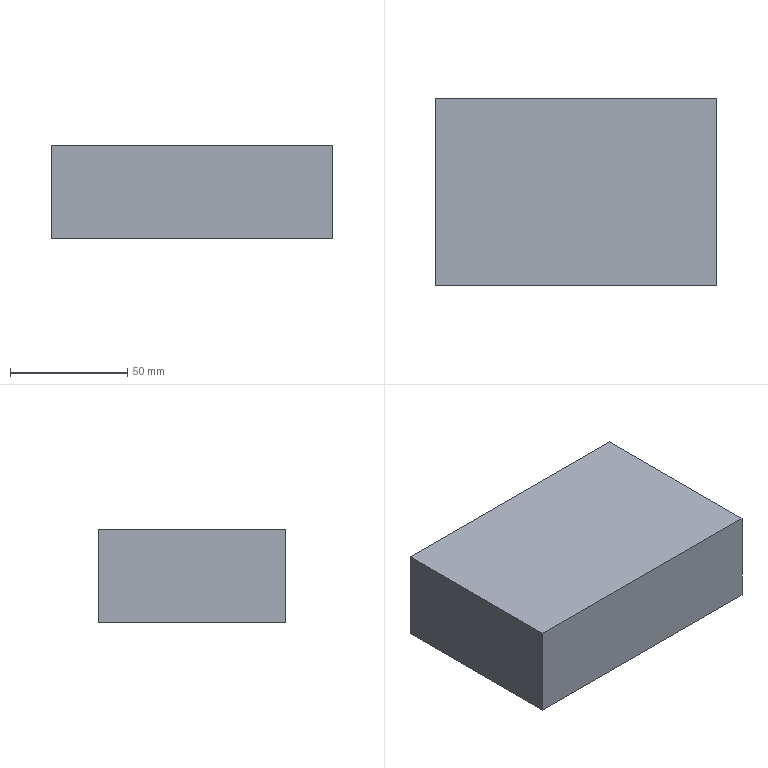Part | SolidWorks | features ICE 2, Extrusion 1 | 1 solid | 11 faces | box 120 x 80 x 40 mm | volume 204000 mm3 | plane 11
STEP:
#1=CARTESIAN_POINT('',(60.,40.,0.));
#2=VERTEX_POINT('',#1);
#3=CARTESIAN_POINT('',(60.,40.,40.));
#4=VERTEX_POINT('',#3);
#5=CARTESIAN_POINT('',(60.,40.,0.));
#6=DIRECTION('',(0.,0.,1.));
#7=VECTOR('',#6,1000.);
#8=LINE('',#5,#7);
#9=EDGE_CURVE('',#2,#4,#8,.T.);
#10=ORIENTED_EDGE('',*,*,#9,.T.);
#11=CARTESIAN_POINT('',(60.,-40.,40.));
#12=VERTEX_POINT('',#11);
#13=CARTESIAN_POINT('',(60.,-40.,40.));
#14=DIRECTION('',(0.,1.,0.));
#15=VECTOR('',#14,1000.);
#16=LINE('',#13,#15);
#17=EDGE_CURVE('',#12,#4,#16,.T.);
#18=ORIENTED_EDGE('',*,*,#17,.F.);
#19=CARTESIAN_POINT('',(60.,-40.,0.));
#20=VERTEX_POINT('',#19);
#21=CARTESIAN_POINT('',(60.,-40.,0.));
#22=DIRECTION('',(0.,0.,1.));
#23=VECTOR('',#22,1000.);
#24=LINE('',#21,#23);
#25=EDGE_CURVE('',#20,#12,#24,.T.);
#26=ORIENTED_EDGE('',*,*,#25,.F.);
#27=CARTESIAN_POINT('',(60.,-40.,0.));
#28=DIRECTION('',(0.,1.,0.));
#29=VECTOR('',#28,1000.);
#30=LINE('',#27,#29);
#31=EDGE_CURVE('',#20,#2,#30,.T.);
#32=ORIENTED_EDGE('',*,*,#31,.T.);
#33=EDGE_LOOP('',(#10,#18,#26,#32));
#34=FACE_OUTER_BOUND('',#33,.T.);
#35=CARTESIAN_POINT('',(60.,-40.,0.));
#36=DIRECTION('',(1.,0.,0.));
#37=DIRECTION('',(0.,0.,-1.));
#38=AXIS2_PLACEMENT_3D('',#35,#36,#37);
#39=PLANE('',#38);
#40=ADVANCED_FACE('',(#34),#39,.T.);
#41=ORIENTED_EDGE('',*,*,#25,.T.);
#42=CARTESIAN_POINT('',(-60.,-40.,40.));
#43=VERTEX_POINT('',#42);
#44=CARTESIAN_POINT('',(-60.,-40.,40.));
#45=DIRECTION('',(1.,0.,0.));
#46=VECTOR('',#45,1000.);
#47=LINE('',#44,#46);
#48=EDGE_CURVE('',#43,#12,#47,.T.);
#49=ORIENTED_EDGE('',*,*,#48,.F.);
#50=CARTESIAN_POINT('',(-60.,-40.,0.));
#51=VERTEX_POINT('',#50);
#52=CARTESIAN_POINT('',(-60.,-40.,0.));
#53=DIRECTION('',(0.,0.,1.));
#54=VECTOR('',#53,1000.);
#55=LINE('',#52,#54);
#56=EDGE_CURVE('',#51,#43,#55,.T.);
#57=ORIENTED_EDGE('',*,*,#56,.F.);
#58=CARTESIAN_POINT('',(-60.,-40.,0.));
#59=DIRECTION('',(1.,0.,0.));
#60=VECTOR('',#59,1000.);
#61=LINE('',#58,#60);
#62=EDGE_CURVE('',#51,#20,#61,.T.);
#63=ORIENTED_EDGE('',*,*,#62,.T.);
#64=EDGE_LOOP('',(#41,#49,#57,#63));
#65=FACE_OUTER_BOUND('',#64,.T.);
#66=CARTESIAN_POINT('',(-60.,-40.,0.));
#67=DIRECTION('',(0.,-1.,0.));
#68=DIRECTION('',(1.,0.,0.));
#69=AXIS2_PLACEMENT_3D('',#66,#67,#68);
#70=PLANE('',#69);
#71=ADVANCED_FACE('',(#65),#70,.T.);
#72=ORIENTED_EDGE('',*,*,#56,.T.);
#73=CARTESIAN_POINT('',(-60.,40.,40.));
#74=VERTEX_POINT('',#73);
#75=CARTESIAN_POINT('',(-60.,40.,40.));
#76=DIRECTION('',(0.,-1.,0.));
#77=VECTOR('',#76,1000.);
#78=LINE('',#75,#77);
#79=EDGE_CURVE('',#74,#43,#78,.T.);
#80=ORIENTED_EDGE('',*,*,#79,.F.);
#81=CARTESIAN_POINT('',(-60.,40.,0.));
#82=VERTEX_POINT('',#81);
#83=CARTESIAN_POINT('',(-60.,40.,0.));
#84=DIRECTION('',(0.,0.,1.));
#85=VECTOR('',#84,1000.);
#86=LINE('',#83,#85);
#87=EDGE_CURVE('',#82,#74,#86,.T.);
#88=ORIENTED_EDGE('',*,*,#87,.F.);
#89=CARTESIAN_POINT('',(-60.,40.,0.));
#90=DIRECTION('',(0.,-1.,0.));
#91=VECTOR('',#90,1000.);
#92=LINE('',#89,#91);
#93=EDGE_CURVE('',#82,#51,#92,.T.);
#94=ORIENTED_EDGE('',*,*,#93,.T.);
#95=EDGE_LOOP('',(#72,#80,#88,#94));
#96=FACE_OUTER_BOUND('',#95,.T.);
#97=CARTESIAN_POINT('',(-60.,40.,0.));
#98=DIRECTION('',(-1.,0.,0.));
#99=DIRECTION('',(0.,-1.,0.));
#100=AXIS2_PLACEMENT_3D('',#97,#98,#99);
#101=PLANE('',#100);
#102=ADVANCED_FACE('',(#96),#101,.T.);
#103=ORIENTED_EDGE('',*,*,#87,.T.);
#104=CARTESIAN_POINT('',(60.,40.,40.));
#105=DIRECTION('',(-1.,0.,0.));
#106=VECTOR('',#105,1000.);
#107=LINE('',#104,#106);
#108=EDGE_CURVE('',#4,#74,#107,.T.);
#109=ORIENTED_EDGE('',*,*,#108,.F.);
#110=ORIENTED_EDGE('',*,*,#9,.F.);
#111=CARTESIAN_POINT('',(60.,40.,0.));
#112=DIRECTION('',(-1.,0.,0.));
#113=VECTOR('',#112,1000.);
#114=LINE('',#111,#113);
#115=EDGE_CURVE('',#2,#82,#114,.T.);
#116=ORIENTED_EDGE('',*,*,#115,.T.);
#117=EDGE_LOOP('',(#103,#109,#110,#116));
#118=FACE_OUTER_BOUND('',#117,.T.);
#119=CARTESIAN_POINT('',(60.,40.,0.));
#120=DIRECTION('',(0.,1.,0.));
#121=DIRECTION('',(-1.,0.,0.));
#122=AXIS2_PLACEMENT_3D('',#119,#120,#121);
#123=PLANE('',#122);
#124=ADVANCED_FACE('',(#118),#123,.T.);
#125=CARTESIAN_POINT('',(50.,-30.,0.));
#126=VERTEX_POINT('',#125);
#127=CARTESIAN_POINT('',(50.,30.,0.));
#128=VERTEX_POINT('',#127);
#129=CARTESIAN_POINT('',(50.,-30.,0.));
#130=DIRECTION('',(0.,1.,0.));
#131=VECTOR('',#130,1000.);
#132=LINE('',#129,#131);
#133=EDGE_CURVE('',#126,#128,#132,.T.);
#134=ORIENTED_EDGE('',*,*,#133,.T.);
#135=CARTESIAN_POINT('',(-50.,30.,0.));
#136=VERTEX_POINT('',#135);
#137=CARTESIAN_POINT('',(50.,30.,0.));
#138=DIRECTION('',(-1.,0.,0.));
#139=VECTOR('',#138,1000.);
#140=LINE('',#137,#139);
#141=EDGE_CURVE('',#128,#136,#140,.T.);
#142=ORIENTED_EDGE('',*,*,#141,.T.);
#143=CARTESIAN_POINT('',(-50.,-30.,0.));
#144=VERTEX_POINT('',#143);
#145=CARTESIAN_POINT('',(-50.,30.,0.));
#146=DIRECTION('',(0.,-1.,0.));
#147=VECTOR('',#146,1000.);
#148=LINE('',#145,#147);
#149=EDGE_CURVE('',#136,#144,#148,.T.);
#150=ORIENTED_EDGE('',*,*,#149,.T.);
#151=CARTESIAN_POINT('',(-50.,-30.,0.));
#152=DIRECTION('',(1.,0.,0.));
#153=VECTOR('',#152,1000.);
#154=LINE('',#151,#153);
#155=EDGE_CURVE('',#144,#126,#154,.T.);
#156=ORIENTED_EDGE('',*,*,#155,.T.);
#157=EDGE_LOOP('',(#134,#142,#150,#156));
#158=FACE_BOUND('',#157,.T.);
#159=ORIENTED_EDGE('',*,*,#31,.F.);
#160=ORIENTED_EDGE('',*,*,#62,.F.);
#161=ORIENTED_EDGE('',*,*,#93,.F.);
#162=ORIENTED_EDGE('',*,*,#115,.F.);
#163=EDGE_LOOP('',(#159,#160,#161,#162));
#164=FACE_OUTER_BOUND('',#163,.T.);
#165=CARTESIAN_POINT('',(0.,0.,0.));
#166=DIRECTION('',(0.,0.,1.));
#167=DIRECTION('',(1.,0.,0.));
#168=AXIS2_PLACEMENT_3D('',#165,#166,#167);
#169=PLANE('',#168);
#170=ADVANCED_FACE('',(#158,#164),#169,.F.);
#171=CARTESIAN_POINT('',(50.,30.,30.));
#172=VERTEX_POINT('',#171);
#173=CARTESIAN_POINT('',(-50.,30.,30.));
#174=VERTEX_POINT('',#173);
#175=CARTESIAN_POINT('',(50.,30.,30.));
#176=DIRECTION('',(-1.,0.,0.));
#177=VECTOR('',#176,1000.);
#178=LINE('',#175,#177);
#179=EDGE_CURVE('',#172,#174,#178,.T.);
#180=ORIENTED_EDGE('',*,*,#179,.T.);
#181=CARTESIAN_POINT('',(-50.,30.,0.));
#182=DIRECTION('',(0.,0.,1.));
#183=VECTOR('',#182,1000.);
#184=LINE('',#181,#183);
#185=EDGE_CURVE('',#136,#174,#184,.T.);
#186=ORIENTED_EDGE('',*,*,#185,.F.);
#187=ORIENTED_EDGE('',*,*,#141,.F.);
#188=CARTESIAN_POINT('',(50.,30.,0.));
#189=DIRECTION('',(0.,0.,1.));
#190=VECTOR('',#189,1000.);
#191=LINE('',#188,#190);
#192=EDGE_CURVE('',#128,#172,#191,.T.);
#193=ORIENTED_EDGE('',*,*,#192,.T.);
#194=EDGE_LOOP('',(#180,#186,#187,#193));
#195=FACE_OUTER_BOUND('',#194,.T.);
#196=CARTESIAN_POINT('',(50.,30.,0.));
#197=DIRECTION('',(0.,1.,0.));
#198=DIRECTION('',(-1.,0.,0.));
#199=AXIS2_PLACEMENT_3D('',#196,#197,#198);
#200=PLANE('',#199);
#201=ADVANCED_FACE('',(#195),#200,.F.);
#202=CARTESIAN_POINT('',(50.,-30.,30.));
#203=VERTEX_POINT('',#202);
#204=CARTESIAN_POINT('',(50.,-30.,30.));
#205=DIRECTION('',(0.,1.,0.));
#206=VECTOR('',#205,1000.);
#207=LINE('',#204,#206);
#208=EDGE_CURVE('',#203,#172,#207,.T.);
#209=ORIENTED_EDGE('',*,*,#208,.T.);
#210=ORIENTED_EDGE('',*,*,#192,.F.);
#211=ORIENTED_EDGE('',*,*,#133,.F.);
#212=CARTESIAN_POINT('',(50.,-30.,0.));
#213=DIRECTION('',(0.,0.,1.));
#214=VECTOR('',#213,1000.);
#215=LINE('',#212,#214);
#216=EDGE_CURVE('',#126,#203,#215,.T.);
#217=ORIENTED_EDGE('',*,*,#216,.T.);
#218=EDGE_LOOP('',(#209,#210,#211,#217));
#219=FACE_OUTER_BOUND('',#218,.T.);
#220=CARTESIAN_POINT('',(50.,-30.,0.));
#221=DIRECTION('',(1.,0.,0.));
#222=DIRECTION('',(0.,0.,-1.));
#223=AXIS2_PLACEMENT_3D('',#220,#221,#222);
#224=PLANE('',#223);
#225=ADVANCED_FACE('',(#219),#224,.F.);
#226=CARTESIAN_POINT('',(-50.,-30.,30.));
#227=VERTEX_POINT('',#226);
#228=CARTESIAN_POINT('',(-50.,-30.,30.));
#229=DIRECTION('',(1.,0.,0.));
#230=VECTOR('',#229,1000.);
#231=LINE('',#228,#230);
#232=EDGE_CURVE('',#227,#203,#231,.T.);
#233=ORIENTED_EDGE('',*,*,#232,.T.);
#234=ORIENTED_EDGE('',*,*,#216,.F.);
#235=ORIENTED_EDGE('',*,*,#155,.F.);
#236=CARTESIAN_POINT('',(-50.,-30.,0.));
#237=DIRECTION('',(0.,0.,1.));
#238=VECTOR('',#237,1000.);
#239=LINE('',#236,#238);
#240=EDGE_CURVE('',#144,#227,#239,.T.);
#241=ORIENTED_EDGE('',*,*,#240,.T.);
#242=EDGE_LOOP('',(#233,#234,#235,#241));
#243=FACE_OUTER_BOUND('',#242,.T.);
#244=CARTESIAN_POINT('',(-50.,-30.,0.));
#245=DIRECTION('',(0.,-1.,0.));
#246=DIRECTION('',(1.,0.,0.));
#247=AXIS2_PLACEMENT_3D('',#244,#245,#246);
#248=PLANE('',#247);
#249=ADVANCED_FACE('',(#243),#248,.F.);
#250=CARTESIAN_POINT('',(-50.,30.,30.));
#251=DIRECTION('',(0.,-1.,0.));
#252=VECTOR('',#251,1000.);
#253=LINE('',#250,#252);
#254=EDGE_CURVE('',#174,#227,#253,.T.);
#255=ORIENTED_EDGE('',*,*,#254,.T.);
#256=ORIENTED_EDGE('',*,*,#240,.F.);
#257=ORIENTED_EDGE('',*,*,#149,.F.);
#258=ORIENTED_EDGE('',*,*,#185,.T.);
#259=EDGE_LOOP('',(#255,#256,#257,#258));
#260=FACE_OUTER_BOUND('',#259,.T.);
#261=CARTESIAN_POINT('',(-50.,30.,0.));
#262=DIRECTION('',(-1.,0.,0.));
#263=DIRECTION('',(0.,0.,1.));
#264=AXIS2_PLACEMENT_3D('',#261,#262,#263);
#265=PLANE('',#264);
#266=ADVANCED_FACE('',(#260),#265,.F.);
#267=ORIENTED_EDGE('',*,*,#179,.F.);
#268=ORIENTED_EDGE('',*,*,#208,.F.);
#269=ORIENTED_EDGE('',*,*,#232,.F.);
#270=ORIENTED_EDGE('',*,*,#254,.F.);
#271=EDGE_LOOP('',(#267,#268,#269,#270));
#272=FACE_OUTER_BOUND('',#271,.T.);
#273=CARTESIAN_POINT('',(0.,0.,30.));
#274=DIRECTION('',(0.,0.,1.));
#275=DIRECTION('',(1.,0.,0.));
#276=AXIS2_PLACEMENT_3D('',#273,#274,#275);
#277=PLANE('',#276);
#278=ADVANCED_FACE('',(#272),#277,.F.);
#279=ORIENTED_EDGE('',*,*,#48,.T.);
#280=ORIENTED_EDGE('',*,*,#17,.T.);
#281=ORIENTED_EDGE('',*,*,#108,.T.);
#282=ORIENTED_EDGE('',*,*,#79,.T.);
#283=EDGE_LOOP('',(#279,#280,#281,#282));
#284=FACE_OUTER_BOUND('',#283,.T.);
#285=CARTESIAN_POINT('',(0.,0.,40.));
#286=DIRECTION('',(0.,0.,1.));
#287=DIRECTION('',(1.,0.,0.));
#288=AXIS2_PLACEMENT_3D('',#285,#286,#287);
#289=PLANE('',#288);
#290=ADVANCED_FACE('',(#284),#289,.T.);
#291=CLOSED_SHELL('',(#40,#71,#102,#124,#170,#201,#225,#249,#266,#278,#290));
#292=MANIFOLD_SOLID_BREP('',#291);
#293=CARTESIAN_POINT('',(0.,0.,0.));
#294=DIRECTION('',(0.,0.,1.));
#295=DIRECTION('',(1.,0.,0.));
#296=AXIS2_PLACEMENT_3D('',#293,#294,#295);
#297=(LENGTH_UNIT()NAMED_UNIT(*)SI_UNIT(.MILLI.,.METRE.));
#298=UNCERTAINTY_MEASURE_WITH_UNIT(LENGTH_MEASURE(0.00001),#297,'','');
#299=(NAMED_UNIT(*)PLANE_ANGLE_UNIT()SI_UNIT($,.RADIAN.));
#300=(NAMED_UNIT(*)SI_UNIT($,.STERADIAN.)SOLID_ANGLE_UNIT());
#301=(GEOMETRIC_REPRESENTATION_CONTEXT(3)GLOBAL_UNCERTAINTY_ASSIGNED_CONTEXT((#298))GLOBAL_UNIT_ASSIGNED_CONTEXT((#297,#299,#300))REPRESENTATION_CONTEXT('',''));
#302=ADVANCED_BREP_SHAPE_REPRESENTATION('',(#292,#296),#301);